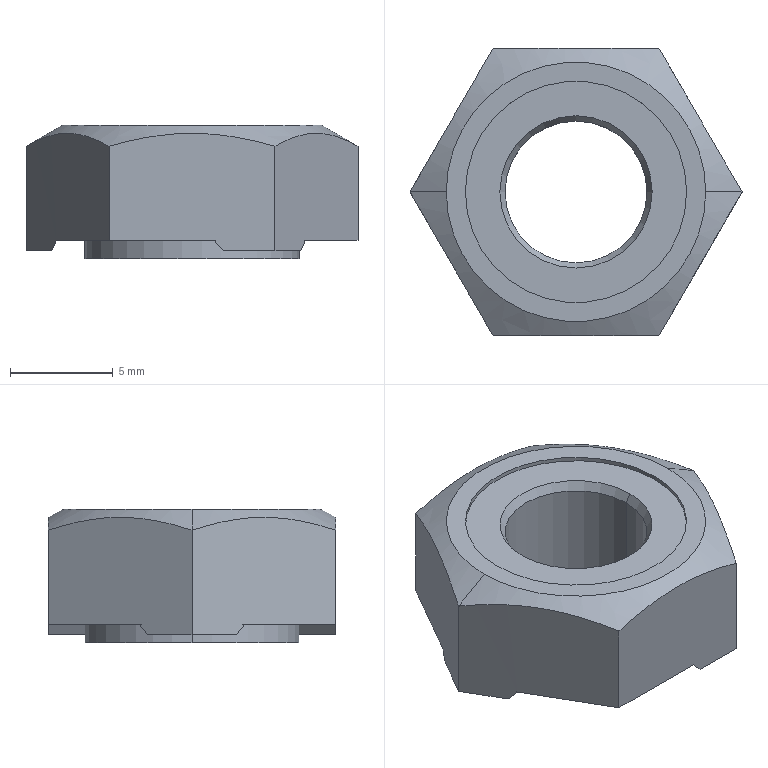Part | STEP file | VD-120102160011A_1_VD-SYL0-5601 | 1 solid | 28 faces | box 16.166 x 14 x 6.5 mm | volume 760.223 mm3 | plane 16 | cone 6 | cylinder 6 | commonest cylinder face diameters 6.917 x2 10.45 x2 10.77 x2
STEP:
#1=CARTESIAN_POINT('',(-3.458,0.,-0.6333));
#2=VERTEX_POINT('',#1);
#3=CARTESIAN_POINT('',(3.458,0.,-0.6333));
#4=VERTEX_POINT('',#3);
#5=CARTESIAN_POINT('',(0.,0.,-0.6333));
#6=DIRECTION('',(0.,0.,-1.));
#7=DIRECTION('',(-1.,0.,0.));
#8=AXIS2_PLACEMENT_3D('',#5,#6,#7);
#9=CIRCLE('',#8,3.458);
#10=EDGE_CURVE('',#2,#4,#9,.T.);
#11=ORIENTED_EDGE('',*,*,#10,.T.);
#12=CARTESIAN_POINT('',(3.709,0.,-0.2));
#13=VERTEX_POINT('',#12);
#14=CARTESIAN_POINT('',(3.709,0.,-0.2));
#15=DIRECTION('',(-0.5,0.,-0.866));
#16=VECTOR('',#15,1000.);
#17=LINE('',#14,#16);
#18=EDGE_CURVE('',#13,#4,#17,.T.);
#19=ORIENTED_EDGE('',*,*,#18,.F.);
#20=CARTESIAN_POINT('',(-3.709,0.,-0.2));
#21=VERTEX_POINT('',#20);
#22=CARTESIAN_POINT('',(0.,0.,-0.2));
#23=DIRECTION('',(0.,0.,-1.));
#24=DIRECTION('',(-1.,0.,0.));
#25=AXIS2_PLACEMENT_3D('',#22,#23,#24);
#26=CIRCLE('',#25,3.709);
#27=EDGE_CURVE('',#21,#13,#26,.T.);
#28=ORIENTED_EDGE('',*,*,#27,.F.);
#29=CARTESIAN_POINT('',(-3.709,0.,-0.2));
#30=DIRECTION('',(0.5,0.,-0.866));
#31=VECTOR('',#30,1000.);
#32=LINE('',#29,#31);
#33=EDGE_CURVE('',#21,#2,#32,.T.);
#34=ORIENTED_EDGE('',*,*,#33,.T.);
#35=EDGE_LOOP('',(#11,#19,#28,#34));
#36=FACE_OUTER_BOUND('',#35,.T.);
#37=CARTESIAN_POINT('',(0.,0.,-0.4167));
#38=DIRECTION('',(0.,0.,1.));
#39=DIRECTION('',(1.,0.,0.));
#40=AXIS2_PLACEMENT_3D('',#37,#38,#39);
#41=CONICAL_SURFACE('',#40,3.584,0.5236);
#42=ADVANCED_FACE('',(#36),#41,.F.);
#43=CARTESIAN_POINT('',(5.291,-4.835,-6.1));
#44=VERTEX_POINT('',#43);
#45=CARTESIAN_POINT('',(4.041,-7.,-6.1));
#46=VERTEX_POINT('',#45);
#47=CARTESIAN_POINT('',(5.291,-4.835,-6.1));
#48=DIRECTION('',(-0.5,-0.866,0.));
#49=VECTOR('',#48,1000.);
#50=LINE('',#47,#49);
#51=EDGE_CURVE('',#44,#46,#50,.T.);
#52=ORIENTED_EDGE('',*,*,#51,.T.);
#53=CARTESIAN_POINT('',(1.541,-7.,-6.1));
#54=VERTEX_POINT('',#53);
#55=CARTESIAN_POINT('',(4.041,-7.,-6.1));
#56=DIRECTION('',(-1.,0.,0.));
#57=VECTOR('',#56,1000.);
#58=LINE('',#55,#57);
#59=EDGE_CURVE('',#46,#54,#58,.T.);
#60=ORIENTED_EDGE('',*,*,#59,.T.);
#61=CARTESIAN_POINT('',(1.541,-7.,-6.1));
#62=DIRECTION('',(0.866,0.5,0.));
#63=VECTOR('',#62,1000.);
#64=LINE('',#61,#63);
#65=EDGE_CURVE('',#54,#44,#64,.T.);
#66=ORIENTED_EDGE('',*,*,#65,.T.);
#67=EDGE_LOOP('',(#52,#60,#66));
#68=FACE_OUTER_BOUND('',#67,.T.);
#69=CARTESIAN_POINT('',(4.041,-7.,-6.1));
#70=DIRECTION('',(0.,0.,-1.));
#71=DIRECTION('',(0.,-1.,0.));
#72=AXIS2_PLACEMENT_3D('',#69,#70,#71);
#73=PLANE('',#72);
#74=ADVANCED_FACE('',(#68),#73,.T.);
#75=CARTESIAN_POINT('',(1.075,-7.,-5.6));
#76=VERTEX_POINT('',#75);
#77=CARTESIAN_POINT('',(5.525,-4.431,-5.6));
#78=VERTEX_POINT('',#77);
#79=CARTESIAN_POINT('',(1.075,-7.,-5.6));
#80=DIRECTION('',(0.866,0.5,0.));
#81=VECTOR('',#80,1000.);
#82=LINE('',#79,#81);
#83=EDGE_CURVE('',#76,#78,#82,.T.);
#84=ORIENTED_EDGE('',*,*,#83,.T.);
#85=CARTESIAN_POINT('',(5.291,-4.835,-6.1));
#86=DIRECTION('',(0.341,0.5907,0.7313));
#87=VECTOR('',#86,1000.);
#88=LINE('',#85,#87);
#89=EDGE_CURVE('',#44,#78,#88,.T.);
#90=ORIENTED_EDGE('',*,*,#89,.F.);
#91=ORIENTED_EDGE('',*,*,#65,.F.);
#92=CARTESIAN_POINT('',(1.075,-7.,-5.6));
#93=DIRECTION('',(0.682,0.,-0.7313));
#94=VECTOR('',#93,1000.);
#95=LINE('',#92,#94);
#96=EDGE_CURVE('',#76,#54,#95,.T.);
#97=ORIENTED_EDGE('',*,*,#96,.F.);
#98=EDGE_LOOP('',(#84,#90,#91,#97));
#99=FACE_OUTER_BOUND('',#98,.T.);
#100=CARTESIAN_POINT('',(1.541,-7.,-6.1));
#101=DIRECTION('',(-0.4532,0.7849,-0.4226));
#102=DIRECTION('',(-0.682,0.,0.7313));
#103=AXIS2_PLACEMENT_3D('',#100,#101,#102);
#104=PLANE('',#103);
#105=ADVANCED_FACE('',(#99),#104,.T.);
#106=CARTESIAN_POINT('',(1.541,7.,-6.1));
#107=VERTEX_POINT('',#106);
#108=CARTESIAN_POINT('',(4.041,7.,-6.1));
#109=VERTEX_POINT('',#108);
#110=CARTESIAN_POINT('',(1.541,7.,-6.1));
#111=DIRECTION('',(1.,0.,0.));
#112=VECTOR('',#111,1000.);
#113=LINE('',#110,#112);
#114=EDGE_CURVE('',#107,#109,#113,.T.);
#115=ORIENTED_EDGE('',*,*,#114,.T.);
#116=CARTESIAN_POINT('',(5.291,4.835,-6.1));
#117=VERTEX_POINT('',#116);
#118=CARTESIAN_POINT('',(4.041,7.,-6.1));
#119=DIRECTION('',(0.5,-0.866,0.));
#120=VECTOR('',#119,1000.);
#121=LINE('',#118,#120);
#122=EDGE_CURVE('',#109,#117,#121,.T.);
#123=ORIENTED_EDGE('',*,*,#122,.T.);
#124=CARTESIAN_POINT('',(5.291,4.835,-6.1));
#125=DIRECTION('',(-0.866,0.5,0.));
#126=VECTOR('',#125,1000.);
#127=LINE('',#124,#126);
#128=EDGE_CURVE('',#117,#107,#127,.T.);
#129=ORIENTED_EDGE('',*,*,#128,.T.);
#130=EDGE_LOOP('',(#115,#123,#129));
#131=FACE_OUTER_BOUND('',#130,.T.);
#132=CARTESIAN_POINT('',(4.041,7.,-6.1));
#133=DIRECTION('',(0.,0.,-1.));
#134=DIRECTION('',(0.,-1.,0.));
#135=AXIS2_PLACEMENT_3D('',#132,#133,#134);
#136=PLANE('',#135);
#137=ADVANCED_FACE('',(#131),#136,.T.);
#138=CARTESIAN_POINT('',(1.075,7.,-5.6));
#139=VERTEX_POINT('',#138);
#140=CARTESIAN_POINT('',(5.525,4.431,-5.6));
#141=VERTEX_POINT('',#140);
#142=CARTESIAN_POINT('',(1.075,7.,-5.6));
#143=DIRECTION('',(0.866,-0.5,0.));
#144=VECTOR('',#143,1000.);
#145=LINE('',#142,#144);
#146=EDGE_CURVE('',#139,#141,#145,.T.);
#147=ORIENTED_EDGE('',*,*,#146,.F.);
#148=CARTESIAN_POINT('',(1.541,7.,-6.1));
#149=DIRECTION('',(-0.682,0.,0.7313));
#150=VECTOR('',#149,1000.);
#151=LINE('',#148,#150);
#152=EDGE_CURVE('',#107,#139,#151,.T.);
#153=ORIENTED_EDGE('',*,*,#152,.F.);
#154=ORIENTED_EDGE('',*,*,#128,.F.);
#155=CARTESIAN_POINT('',(5.291,4.835,-6.1));
#156=DIRECTION('',(0.341,-0.5907,0.7313));
#157=VECTOR('',#156,1000.);
#158=LINE('',#155,#157);
#159=EDGE_CURVE('',#117,#141,#158,.T.);
#160=ORIENTED_EDGE('',*,*,#159,.T.);
#161=EDGE_LOOP('',(#147,#153,#154,#160));
#162=FACE_OUTER_BOUND('',#161,.T.);
#163=CARTESIAN_POINT('',(5.291,4.835,-6.1));
#164=DIRECTION('',(-0.4532,-0.7849,-0.4226));
#165=DIRECTION('',(-0.866,0.5,0.));
#166=AXIS2_PLACEMENT_3D('',#163,#164,#165);
#167=PLANE('',#166);
#168=ADVANCED_FACE('',(#162),#167,.T.);
#169=CARTESIAN_POINT('',(-6.6,2.569,-5.6));
#170=VERTEX_POINT('',#169);
#171=CARTESIAN_POINT('',(-6.6,-2.569,-5.6));
#172=VERTEX_POINT('',#171);
#173=CARTESIAN_POINT('',(-6.6,2.569,-5.6));
#174=DIRECTION('',(0.,-1.,0.));
#175=VECTOR('',#174,1000.);
#176=LINE('',#173,#175);
#177=EDGE_CURVE('',#170,#172,#176,.T.);
#178=ORIENTED_EDGE('',*,*,#177,.T.);
#179=CARTESIAN_POINT('',(-6.833,-2.165,-6.1));
#180=VERTEX_POINT('',#179);
#181=CARTESIAN_POINT('',(-6.6,-2.569,-5.6));
#182=DIRECTION('',(-0.341,0.5907,-0.7313));
#183=VECTOR('',#182,1000.);
#184=LINE('',#181,#183);
#185=EDGE_CURVE('',#172,#180,#184,.T.);
#186=ORIENTED_EDGE('',*,*,#185,.T.);
#187=CARTESIAN_POINT('',(-6.833,2.165,-6.1));
#188=VERTEX_POINT('',#187);
#189=CARTESIAN_POINT('',(-6.833,2.165,-6.1));
#190=DIRECTION('',(0.,-1.,0.));
#191=VECTOR('',#190,1000.);
#192=LINE('',#189,#191);
#193=EDGE_CURVE('',#188,#180,#192,.T.);
#194=ORIENTED_EDGE('',*,*,#193,.F.);
#195=CARTESIAN_POINT('',(-6.833,2.165,-6.1));
#196=DIRECTION('',(0.341,0.5907,0.7313));
#197=VECTOR('',#196,1000.);
#198=LINE('',#195,#197);
#199=EDGE_CURVE('',#188,#170,#198,.T.);
#200=ORIENTED_EDGE('',*,*,#199,.T.);
#201=EDGE_LOOP('',(#178,#186,#194,#200));
#202=FACE_OUTER_BOUND('',#201,.T.);
#203=CARTESIAN_POINT('',(-6.833,2.165,-6.1));
#204=DIRECTION('',(0.9063,0.,-0.4226));
#205=DIRECTION('',(0.,-1.,0.));
#206=AXIS2_PLACEMENT_3D('',#203,#204,#205);
#207=PLANE('',#206);
#208=ADVANCED_FACE('',(#202),#207,.T.);
#209=CARTESIAN_POINT('',(-8.083,0.,-6.1));
#210=VERTEX_POINT('',#209);
#211=CARTESIAN_POINT('',(-6.833,-2.165,-6.1));
#212=DIRECTION('',(-0.5,0.866,0.));
#213=VECTOR('',#212,1000.);
#214=LINE('',#211,#213);
#215=EDGE_CURVE('',#180,#210,#214,.T.);
#216=ORIENTED_EDGE('',*,*,#215,.T.);
#217=CARTESIAN_POINT('',(-8.083,0.,-6.1));
#218=DIRECTION('',(0.5,0.866,0.));
#219=VECTOR('',#218,1000.);
#220=LINE('',#217,#219);
#221=EDGE_CURVE('',#210,#188,#220,.T.);
#222=ORIENTED_EDGE('',*,*,#221,.T.);
#223=ORIENTED_EDGE('',*,*,#193,.T.);
#224=EDGE_LOOP('',(#216,#222,#223));
#225=FACE_OUTER_BOUND('',#224,.T.);
#226=CARTESIAN_POINT('',(-8.083,0.,-6.1));
#227=DIRECTION('',(0.,0.,-1.));
#228=DIRECTION('',(0.,-1.,0.));
#229=AXIS2_PLACEMENT_3D('',#226,#227,#228);
#230=PLANE('',#229);
#231=ADVANCED_FACE('',(#225),#230,.T.);
#232=CARTESIAN_POINT('',(-4.041,7.,-1.021));
#233=VERTEX_POINT('',#232);
#234=CARTESIAN_POINT('',(-4.041,7.,-5.6));
#235=VERTEX_POINT('',#234);
#236=CARTESIAN_POINT('',(-4.041,7.,-1.021));
#237=DIRECTION('',(0.,0.,-1.));
#238=VECTOR('',#237,1000.);
#239=LINE('',#236,#238);
#240=EDGE_CURVE('',#233,#235,#239,.T.);
#241=ORIENTED_EDGE('',*,*,#240,.T.);
#242=CARTESIAN_POINT('',(-6.6,2.569,-5.6));
#243=DIRECTION('',(0.5,0.866,0.));
#244=VECTOR('',#243,1000.);
#245=LINE('',#242,#244);
#246=EDGE_CURVE('',#170,#235,#245,.T.);
#247=ORIENTED_EDGE('',*,*,#246,.F.);
#248=ORIENTED_EDGE('',*,*,#199,.F.);
#249=ORIENTED_EDGE('',*,*,#221,.F.);
#250=CARTESIAN_POINT('',(-8.083,0.,-1.021));
#251=VERTEX_POINT('',#250);
#252=CARTESIAN_POINT('',(-8.083,0.,-6.1));
#253=DIRECTION('',(0.,0.,1.));
#254=VECTOR('',#253,1000.);
#255=LINE('',#252,#254);
#256=EDGE_CURVE('',#210,#251,#255,.T.);
#257=ORIENTED_EDGE('',*,*,#256,.T.);
#258=CARTESIAN_POINT('',(-4.041,7.,-1.021));
#259=CARTESIAN_POINT('',(-4.218,6.695,-0.9189));
#260=CARTESIAN_POINT('',(-4.39,6.396,-0.8294));
#261=CARTESIAN_POINT('',(-4.644,5.955,-0.7134));
#262=CARTESIAN_POINT('',(-4.729,5.809,-0.6778));
#263=CARTESIAN_POINT('',(-4.855,5.591,-0.629));
#264=CARTESIAN_POINT('',(-4.897,5.519,-0.6134));
#265=CARTESIAN_POINT('',(-4.98,5.374,-0.5839));
#266=CARTESIAN_POINT('',(-5.021,5.303,-0.5702));
#267=CARTESIAN_POINT('',(-5.404,4.64,-0.449));
#268=CARTESIAN_POINT('',(-5.737,4.063,-0.3948));
#269=CARTESIAN_POINT('',(-6.234,3.203,-0.3958));
#270=CARTESIAN_POINT('',(-6.399,2.917,-0.4097));
#271=CARTESIAN_POINT('',(-6.648,2.485,-0.4507));
#272=CARTESIAN_POINT('',(-6.731,2.341,-0.4676));
#273=CARTESIAN_POINT('',(-6.857,2.124,-0.498));
#274=CARTESIAN_POINT('',(-6.898,2.052,-0.509));
#275=CARTESIAN_POINT('',(-6.982,1.906,-0.5326));
#276=CARTESIAN_POINT('',(-7.025,1.832,-0.5455));
#277=CARTESIAN_POINT('',(-7.399,1.185,-0.6644));
#278=CARTESIAN_POINT('',(-7.732,0.6069,-0.8184));
#279=CARTESIAN_POINT('',(-8.083,0.,-1.021));
#280=B_SPLINE_CURVE_WITH_KNOTS('',3,(#258,#259,#260,#261,#262,#263,#264,#265,#266,#267,#268,#269,#270,#271,#272,#273,#274,#275,#276,#277,#278,#279),.UNSPECIFIED.,.F.,.F.,(4,2,2,2,2,2,2,2,2,2,4),(0.,0.125,0.1875,0.2187,0.25,0.5,0.625,0.6875,0.7188,0.75,1.),.UNSPECIFIED.);
#281=EDGE_CURVE('',#233,#251,#280,.T.);
#282=ORIENTED_EDGE('',*,*,#281,.F.);
#283=EDGE_LOOP('',(#241,#247,#248,#249,#257,#282));
#284=FACE_OUTER_BOUND('',#283,.T.);
#285=CARTESIAN_POINT('',(-4.041,7.,-6.5));
#286=DIRECTION('',(-0.866,0.5,0.));
#287=DIRECTION('',(0.,0.,1.));
#288=AXIS2_PLACEMENT_3D('',#285,#286,#287);
#289=PLANE('',#288);
#290=ADVANCED_FACE('',(#284),#289,.T.);
#291=CARTESIAN_POINT('',(4.041,7.,-1.021));
#292=VERTEX_POINT('',#291);
#293=CARTESIAN_POINT('',(4.041,7.,-1.021));
#294=DIRECTION('',(0.,0.,-1.));
#295=VECTOR('',#294,1000.);
#296=LINE('',#293,#295);
#297=EDGE_CURVE('',#292,#109,#296,.T.);
#298=ORIENTED_EDGE('',*,*,#297,.T.);
#299=ORIENTED_EDGE('',*,*,#114,.F.);
#300=ORIENTED_EDGE('',*,*,#152,.T.);
#301=CARTESIAN_POINT('',(1.075,7.,-5.6));
#302=DIRECTION('',(-1.,0.,0.));
#303=VECTOR('',#302,1000.);
#304=LINE('',#301,#303);
#305=EDGE_CURVE('',#139,#235,#304,.T.);
#306=ORIENTED_EDGE('',*,*,#305,.T.);
#307=ORIENTED_EDGE('',*,*,#240,.F.);
#308=CARTESIAN_POINT('',(4.041,7.,-1.021));
#309=CARTESIAN_POINT('',(3.689,7.,-0.9189));
#310=CARTESIAN_POINT('',(3.345,7.,-0.8294));
#311=CARTESIAN_POINT('',(2.835,7.,-0.7134));
#312=CARTESIAN_POINT('',(2.667,7.,-0.6778));
#313=CARTESIAN_POINT('',(2.415,7.,-0.629));
#314=CARTESIAN_POINT('',(2.331,7.,-0.6134));
#315=CARTESIAN_POINT('',(2.164,7.,-0.5839));
#316=CARTESIAN_POINT('',(2.082,7.,-0.5702));
#317=CARTESIAN_POINT('',(1.316,7.,-0.449));
#318=CARTESIAN_POINT('',(0.6504,7.,-0.3948));
#319=CARTESIAN_POINT('',(-0.3433,7.,-0.3958));
#320=CARTESIAN_POINT('',(-0.6728,7.,-0.4097));
#321=CARTESIAN_POINT('',(-1.172,7.,-0.4507));
#322=CARTESIAN_POINT('',(-1.338,7.,-0.4676));
#323=CARTESIAN_POINT('',(-1.589,7.,-0.498));
#324=CARTESIAN_POINT('',(-1.673,7.,-0.509));
#325=CARTESIAN_POINT('',(-1.84,7.,-0.5326));
#326=CARTESIAN_POINT('',(-1.926,7.,-0.5455));
#327=CARTESIAN_POINT('',(-2.673,7.,-0.6644));
#328=CARTESIAN_POINT('',(-3.341,7.,-0.8184));
#329=CARTESIAN_POINT('',(-4.041,7.,-1.021));
#330=B_SPLINE_CURVE_WITH_KNOTS('',3,(#308,#309,#310,#311,#312,#313,#314,#315,#316,#317,#318,#319,#320,#321,#322,#323,#324,#325,#326,#327,#328,#329),.UNSPECIFIED.,.F.,.F.,(4,2,2,2,2,2,2,2,2,2,4),(0.,0.125,0.1875,0.2188,0.25,0.5,0.625,0.6875,0.7188,0.75,1.),.UNSPECIFIED.);
#331=EDGE_CURVE('',#292,#233,#330,.T.);
#332=ORIENTED_EDGE('',*,*,#331,.F.);
#333=EDGE_LOOP('',(#298,#299,#300,#306,#307,#332));
#334=FACE_OUTER_BOUND('',#333,.T.);
#335=CARTESIAN_POINT('',(4.041,7.,-6.5));
#336=DIRECTION('',(0.,1.,0.));
#337=DIRECTION('',(1.,0.,0.));
#338=AXIS2_PLACEMENT_3D('',#335,#336,#337);
#339=PLANE('',#338);
#340=ADVANCED_FACE('',(#334),#339,.T.);
#341=CARTESIAN_POINT('',(8.083,0.,-1.021));
#342=VERTEX_POINT('',#341);
#343=CARTESIAN_POINT('',(8.083,0.,-5.6));
#344=VERTEX_POINT('',#343);
#345=CARTESIAN_POINT('',(8.083,0.,-1.021));
#346=DIRECTION('',(0.,0.,-1.));
#347=VECTOR('',#346,1000.);
#348=LINE('',#345,#347);
#349=EDGE_CURVE('',#342,#344,#348,.T.);
#350=ORIENTED_EDGE('',*,*,#349,.T.);
#351=CARTESIAN_POINT('',(5.525,4.431,-5.6));
#352=DIRECTION('',(0.5,-0.866,0.));
#353=VECTOR('',#352,1000.);
#354=LINE('',#351,#353);
#355=EDGE_CURVE('',#141,#344,#354,.T.);
#356=ORIENTED_EDGE('',*,*,#355,.F.);
#357=ORIENTED_EDGE('',*,*,#159,.F.);
#358=ORIENTED_EDGE('',*,*,#122,.F.);
#359=ORIENTED_EDGE('',*,*,#297,.F.);
#360=CARTESIAN_POINT('',(8.083,0.,-1.021));
#361=CARTESIAN_POINT('',(7.907,0.3053,-0.9189));
#362=CARTESIAN_POINT('',(7.734,0.6035,-0.8294));
#363=CARTESIAN_POINT('',(7.48,1.044,-0.7134));
#364=CARTESIAN_POINT('',(7.395,1.19,-0.6778));
#365=CARTESIAN_POINT('',(7.27,1.409,-0.629));
#366=CARTESIAN_POINT('',(7.228,1.481,-0.6134));
#367=CARTESIAN_POINT('',(7.144,1.626,-0.5839));
#368=CARTESIAN_POINT('',(7.103,1.697,-0.5702));
#369=CARTESIAN_POINT('',(6.72,2.36,-0.449));
#370=CARTESIAN_POINT('',(6.387,2.937,-0.3948));
#371=CARTESIAN_POINT('',(5.89,3.797,-0.3958));
#372=CARTESIAN_POINT('',(5.726,4.083,-0.4097));
#373=CARTESIAN_POINT('',(5.476,4.515,-0.4507));
#374=CARTESIAN_POINT('',(5.393,4.659,-0.4676));
#375=CARTESIAN_POINT('',(5.268,4.876,-0.498));
#376=CARTESIAN_POINT('',(5.226,4.948,-0.509));
#377=CARTESIAN_POINT('',(5.142,5.094,-0.5326));
#378=CARTESIAN_POINT('',(5.099,5.168,-0.5455));
#379=CARTESIAN_POINT('',(4.726,5.815,-0.6644));
#380=CARTESIAN_POINT('',(4.392,6.393,-0.8184));
#381=CARTESIAN_POINT('',(4.041,7.,-1.021));
#382=B_SPLINE_CURVE_WITH_KNOTS('',3,(#360,#361,#362,#363,#364,#365,#366,#367,#368,#369,#370,#371,#372,#373,#374,#375,#376,#377,#378,#379,#380,#381),.UNSPECIFIED.,.F.,.F.,(4,2,2,2,2,2,2,2,2,2,4),(0.,0.125,0.1875,0.2188,0.25,0.5,0.625,0.6875,0.7188,0.75,1.),.UNSPECIFIED.);
#383=EDGE_CURVE('',#342,#292,#382,.T.);
#384=ORIENTED_EDGE('',*,*,#383,.F.);
#385=EDGE_LOOP('',(#350,#356,#357,#358,#359,#384));
#386=FACE_OUTER_BOUND('',#385,.T.);
#387=CARTESIAN_POINT('',(8.083,0.,-6.5));
#388=DIRECTION('',(0.866,0.5,0.));
#389=DIRECTION('',(0.,0.,-1.));
#390=AXIS2_PLACEMENT_3D('',#387,#388,#389);
#391=PLANE('',#390);
#392=ADVANCED_FACE('',(#386),#391,.T.);
#393=CARTESIAN_POINT('',(4.041,-7.,-1.021));
#394=VERTEX_POINT('',#393);
#395=CARTESIAN_POINT('',(4.041,-7.,-1.021));
#396=DIRECTION('',(0.,0.,-1.));
#397=VECTOR('',#396,1000.);
#398=LINE('',#395,#397);
#399=EDGE_CURVE('',#394,#46,#398,.T.);
#400=ORIENTED_EDGE('',*,*,#399,.T.);
#401=ORIENTED_EDGE('',*,*,#51,.F.);
#402=ORIENTED_EDGE('',*,*,#89,.T.);
#403=CARTESIAN_POINT('',(8.083,0.,-5.6));
#404=DIRECTION('',(-0.5,-0.866,0.));
#405=VECTOR('',#404,1000.);
#406=LINE('',#403,#405);
#407=EDGE_CURVE('',#344,#78,#406,.T.);
#408=ORIENTED_EDGE('',*,*,#407,.F.);
#409=ORIENTED_EDGE('',*,*,#349,.F.);
#410=CARTESIAN_POINT('',(4.041,-7.,-1.021));
#411=CARTESIAN_POINT('',(4.218,-6.695,-0.9189));
#412=CARTESIAN_POINT('',(4.39,-6.396,-0.8294));
#413=CARTESIAN_POINT('',(4.644,-5.955,-0.7134));
#414=CARTESIAN_POINT('',(4.729,-5.809,-0.6778));
#415=CARTESIAN_POINT('',(4.855,-5.591,-0.629));
#416=CARTESIAN_POINT('',(4.897,-5.519,-0.6134));
#417=CARTESIAN_POINT('',(4.98,-5.374,-0.5839));
#418=CARTESIAN_POINT('',(5.021,-5.303,-0.5702));
#419=CARTESIAN_POINT('',(5.404,-4.64,-0.449));
#420=CARTESIAN_POINT('',(5.737,-4.063,-0.3948));
#421=CARTESIAN_POINT('',(6.234,-3.203,-0.3958));
#422=CARTESIAN_POINT('',(6.399,-2.917,-0.4097));
#423=CARTESIAN_POINT('',(6.648,-2.485,-0.4507));
#424=CARTESIAN_POINT('',(6.731,-2.341,-0.4676));
#425=CARTESIAN_POINT('',(6.857,-2.124,-0.498));
#426=CARTESIAN_POINT('',(6.898,-2.052,-0.509));
#427=CARTESIAN_POINT('',(6.982,-1.906,-0.5326));
#428=CARTESIAN_POINT('',(7.025,-1.832,-0.5455));
#429=CARTESIAN_POINT('',(7.399,-1.185,-0.6644));
#430=CARTESIAN_POINT('',(7.732,-0.6069,-0.8184));
#431=CARTESIAN_POINT('',(8.083,0.,-1.021));
#432=B_SPLINE_CURVE_WITH_KNOTS('',3,(#410,#411,#412,#413,#414,#415,#416,#417,#418,#419,#420,#421,#422,#423,#424,#425,#426,#427,#428,#429,#430,#431),.UNSPECIFIED.,.F.,.F.,(4,2,2,2,2,2,2,2,2,2,4),(0.,0.125,0.1875,0.2188,0.25,0.5,0.625,0.6875,0.7188,0.75,1.),.UNSPECIFIED.);
#433=EDGE_CURVE('',#394,#342,#432,.T.);
#434=ORIENTED_EDGE('',*,*,#433,.F.);
#435=EDGE_LOOP('',(#400,#401,#402,#408,#409,#434));
#436=FACE_OUTER_BOUND('',#435,.T.);
#437=CARTESIAN_POINT('',(4.041,-7.,-6.5));
#438=DIRECTION('',(0.866,-0.5,0.));
#439=DIRECTION('',(0.,0.,-1.));
#440=AXIS2_PLACEMENT_3D('',#437,#438,#439);
#441=PLANE('',#440);
#442=ADVANCED_FACE('',(#436),#441,.T.);
#443=CARTESIAN_POINT('',(-4.041,-7.,-1.021));
#444=VERTEX_POINT('',#443);
#445=CARTESIAN_POINT('',(-4.041,-7.,-5.6));
#446=VERTEX_POINT('',#445);
#447=CARTESIAN_POINT('',(-4.041,-7.,-1.021));
#448=DIRECTION('',(0.,0.,-1.));
#449=VECTOR('',#448,1000.);
#450=LINE('',#447,#449);
#451=EDGE_CURVE('',#444,#446,#450,.T.);
#452=ORIENTED_EDGE('',*,*,#451,.T.);
#453=CARTESIAN_POINT('',(-4.041,-7.,-5.6));
#454=DIRECTION('',(1.,0.,0.));
#455=VECTOR('',#454,1000.);
#456=LINE('',#453,#455);
#457=EDGE_CURVE('',#446,#76,#456,.T.);
#458=ORIENTED_EDGE('',*,*,#457,.T.);
#459=ORIENTED_EDGE('',*,*,#96,.T.);
#460=ORIENTED_EDGE('',*,*,#59,.F.);
#461=ORIENTED_EDGE('',*,*,#399,.F.);
#462=CARTESIAN_POINT('',(-4.041,-7.,-1.021));
#463=CARTESIAN_POINT('',(-3.689,-7.,-0.9189));
#464=CARTESIAN_POINT('',(-3.345,-7.,-0.8294));
#465=CARTESIAN_POINT('',(-2.835,-7.,-0.7134));
#466=CARTESIAN_POINT('',(-2.667,-7.,-0.6778));
#467=CARTESIAN_POINT('',(-2.415,-7.,-0.629));
#468=CARTESIAN_POINT('',(-2.331,-7.,-0.6134));
#469=CARTESIAN_POINT('',(-2.164,-7.,-0.5839));
#470=CARTESIAN_POINT('',(-2.082,-7.,-0.5702));
#471=CARTESIAN_POINT('',(-1.316,-7.,-0.449));
#472=CARTESIAN_POINT('',(-0.6504,-7.,-0.3948));
#473=CARTESIAN_POINT('',(0.3433,-7.,-0.3958));
#474=CARTESIAN_POINT('',(0.6728,-7.,-0.4097));
#475=CARTESIAN_POINT('',(1.172,-7.,-0.4507));
#476=CARTESIAN_POINT('',(1.338,-7.,-0.4676));
#477=CARTESIAN_POINT('',(1.589,-7.,-0.498));
#478=CARTESIAN_POINT('',(1.673,-7.,-0.509));
#479=CARTESIAN_POINT('',(1.84,-7.,-0.5326));
#480=CARTESIAN_POINT('',(1.926,-7.,-0.5455));
#481=CARTESIAN_POINT('',(2.673,-7.,-0.6644));
#482=CARTESIAN_POINT('',(3.341,-7.,-0.8184));
#483=CARTESIAN_POINT('',(4.041,-7.,-1.021));
#484=B_SPLINE_CURVE_WITH_KNOTS('',3,(#462,#463,#464,#465,#466,#467,#468,#469,#470,#471,#472,#473,#474,#475,#476,#477,#478,#479,#480,#481,#482,#483),.UNSPECIFIED.,.F.,.F.,(4,2,2,2,2,2,2,2,2,2,4),(0.,0.125,0.1875,0.2188,0.25,0.5,0.625,0.6875,0.7188,0.75,1.),.UNSPECIFIED.);
#485=EDGE_CURVE('',#444,#394,#484,.T.);
#486=ORIENTED_EDGE('',*,*,#485,.F.);
#487=EDGE_LOOP('',(#452,#458,#459,#460,#461,#486));
#488=FACE_OUTER_BOUND('',#487,.T.);
#489=CARTESIAN_POINT('',(-4.041,-7.,-6.5));
#490=DIRECTION('',(0.,-1.,0.));
#491=DIRECTION('',(0.,0.,-1.));
#492=AXIS2_PLACEMENT_3D('',#489,#490,#491);
#493=PLANE('',#492);
#494=ADVANCED_FACE('',(#488),#493,.T.);
#495=CARTESIAN_POINT('',(5.225,0.,-5.6));
#496=VERTEX_POINT('',#495);
#497=CARTESIAN_POINT('',(-5.225,0.,-5.6));
#498=VERTEX_POINT('',#497);
#499=CARTESIAN_POINT('',(0.,0.,-5.6));
#500=DIRECTION('',(0.,0.,1.));
#501=DIRECTION('',(1.,0.,0.));
#502=AXIS2_PLACEMENT_3D('',#499,#500,#501);
#503=CIRCLE('',#502,5.225);
#504=EDGE_CURVE('',#496,#498,#503,.T.);
#505=ORIENTED_EDGE('',*,*,#504,.T.);
#506=CARTESIAN_POINT('',(0.,0.,-5.6));
#507=DIRECTION('',(0.,0.,1.));
#508=DIRECTION('',(-1.,0.,0.));
#509=AXIS2_PLACEMENT_3D('',#506,#507,#508);
#510=CIRCLE('',#509,5.225);
#511=EDGE_CURVE('',#498,#496,#510,.T.);
#512=ORIENTED_EDGE('',*,*,#511,.T.);
#513=EDGE_LOOP('',(#505,#512));
#514=FACE_BOUND('',#513,.T.);
#515=CARTESIAN_POINT('',(-4.041,-7.,-5.6));
#516=DIRECTION('',(-0.5,0.866,0.));
#517=VECTOR('',#516,1000.);
#518=LINE('',#515,#517);
#519=EDGE_CURVE('',#446,#172,#518,.T.);
#520=ORIENTED_EDGE('',*,*,#519,.T.);
#521=ORIENTED_EDGE('',*,*,#177,.F.);
#522=ORIENTED_EDGE('',*,*,#246,.T.);
#523=ORIENTED_EDGE('',*,*,#305,.F.);
#524=ORIENTED_EDGE('',*,*,#146,.T.);
#525=ORIENTED_EDGE('',*,*,#355,.T.);
#526=ORIENTED_EDGE('',*,*,#407,.T.);
#527=ORIENTED_EDGE('',*,*,#83,.F.);
#528=ORIENTED_EDGE('',*,*,#457,.F.);
#529=EDGE_LOOP('',(#520,#521,#522,#523,#524,#525,#526,#527,#528));
#530=FACE_OUTER_BOUND('',#529,.T.);
#531=CARTESIAN_POINT('',(0.,0.,-5.6));
#532=DIRECTION('',(0.,0.,-1.));
#533=DIRECTION('',(0.,-1.,0.));
#534=AXIS2_PLACEMENT_3D('',#531,#532,#533);
#535=PLANE('',#534);
#536=ADVANCED_FACE('',(#514,#530),#535,.T.);
#537=CARTESIAN_POINT('',(5.225,0.,-6.5));
#538=VERTEX_POINT('',#537);
#539=CARTESIAN_POINT('',(5.225,0.,-6.5));
#540=DIRECTION('',(0.,0.,1.));
#541=VECTOR('',#540,1000.);
#542=LINE('',#539,#541);
#543=EDGE_CURVE('',#538,#496,#542,.T.);
#544=ORIENTED_EDGE('',*,*,#543,.F.);
#545=CARTESIAN_POINT('',(-5.225,0.,-6.5));
#546=VERTEX_POINT('',#545);
#547=CARTESIAN_POINT('',(0.,0.,-6.5));
#548=DIRECTION('',(0.,0.,-1.));
#549=DIRECTION('',(-1.,0.,0.));
#550=AXIS2_PLACEMENT_3D('',#547,#548,#549);
#551=CIRCLE('',#550,5.225);
#552=EDGE_CURVE('',#546,#538,#551,.T.);
#553=ORIENTED_EDGE('',*,*,#552,.F.);
#554=CARTESIAN_POINT('',(-5.225,0.,-6.5));
#555=DIRECTION('',(0.,0.,1.));
#556=VECTOR('',#555,1000.);
#557=LINE('',#554,#556);
#558=EDGE_CURVE('',#546,#498,#557,.T.);
#559=ORIENTED_EDGE('',*,*,#558,.T.);
#560=ORIENTED_EDGE('',*,*,#504,.F.);
#561=EDGE_LOOP('',(#544,#553,#559,#560));
#562=FACE_OUTER_BOUND('',#561,.T.);
#563=CARTESIAN_POINT('',(0.,0.,-5.6));
#564=DIRECTION('',(0.,0.,-1.));
#565=DIRECTION('',(-1.,0.,0.));
#566=AXIS2_PLACEMENT_3D('',#563,#564,#565);
#567=CYLINDRICAL_SURFACE('',#566,5.225);
#568=ADVANCED_FACE('',(#562),#567,.T.);
#569=ORIENTED_EDGE('',*,*,#511,.F.);
#570=ORIENTED_EDGE('',*,*,#558,.F.);
#571=CARTESIAN_POINT('',(0.,0.,-6.5));
#572=DIRECTION('',(0.,0.,-1.));
#573=DIRECTION('',(1.,0.,0.));
#574=AXIS2_PLACEMENT_3D('',#571,#572,#573);
#575=CIRCLE('',#574,5.225);
#576=EDGE_CURVE('',#538,#546,#575,.T.);
#577=ORIENTED_EDGE('',*,*,#576,.F.);
#578=ORIENTED_EDGE('',*,*,#543,.T.);
#579=EDGE_LOOP('',(#569,#570,#577,#578));
#580=FACE_OUTER_BOUND('',#579,.T.);
#581=CARTESIAN_POINT('',(0.,0.,-5.6));
#582=DIRECTION('',(0.,0.,-1.));
#583=DIRECTION('',(-1.,0.,0.));
#584=AXIS2_PLACEMENT_3D('',#581,#582,#583);
#585=CYLINDRICAL_SURFACE('',#584,5.225);
#586=ADVANCED_FACE('',(#580),#585,.T.);
#587=CARTESIAN_POINT('',(3.892,0.,-6.5));
#588=VERTEX_POINT('',#587);
#589=CARTESIAN_POINT('',(-3.892,0.,-6.5));
#590=VERTEX_POINT('',#589);
#591=CARTESIAN_POINT('',(0.,0.,-6.5));
#592=DIRECTION('',(0.,0.,1.));
#593=DIRECTION('',(1.,0.,0.));
#594=AXIS2_PLACEMENT_3D('',#591,#592,#593);
#595=CIRCLE('',#594,3.892);
#596=EDGE_CURVE('',#588,#590,#595,.T.);
#597=ORIENTED_EDGE('',*,*,#596,.T.);
#598=CARTESIAN_POINT('',(0.,0.,-6.5));
#599=DIRECTION('',(0.,0.,1.));
#600=DIRECTION('',(-1.,0.,0.));
#601=AXIS2_PLACEMENT_3D('',#598,#599,#600);
#602=CIRCLE('',#601,3.892);
#603=EDGE_CURVE('',#590,#588,#602,.T.);
#604=ORIENTED_EDGE('',*,*,#603,.T.);
#605=EDGE_LOOP('',(#597,#604));
#606=FACE_BOUND('',#605,.T.);
#607=ORIENTED_EDGE('',*,*,#552,.T.);
#608=ORIENTED_EDGE('',*,*,#576,.T.);
#609=EDGE_LOOP('',(#607,#608));
#610=FACE_OUTER_BOUND('',#609,.T.);
#611=CARTESIAN_POINT('',(-4.041,-7.,-6.5));
#612=DIRECTION('',(0.,0.,-1.));
#613=DIRECTION('',(0.,-1.,0.));
#614=AXIS2_PLACEMENT_3D('',#611,#612,#613);
#615=PLANE('',#614);
#616=ADVANCED_FACE('',(#606,#610),#615,.T.);
#617=CARTESIAN_POINT('',(3.459,0.,-6.25));
#618=VERTEX_POINT('',#617);
#619=CARTESIAN_POINT('',(3.892,0.,-6.5));
#620=DIRECTION('',(-0.866,0.,0.5));
#621=VECTOR('',#620,1000.);
#622=LINE('',#619,#621);
#623=EDGE_CURVE('',#588,#618,#622,.T.);
#624=ORIENTED_EDGE('',*,*,#623,.F.);
#625=ORIENTED_EDGE('',*,*,#603,.F.);
#626=CARTESIAN_POINT('',(-3.459,0.,-6.25));
#627=VERTEX_POINT('',#626);
#628=CARTESIAN_POINT('',(-3.892,0.,-6.5));
#629=DIRECTION('',(0.866,0.,0.5));
#630=VECTOR('',#629,1000.);
#631=LINE('',#628,#630);
#632=EDGE_CURVE('',#590,#627,#631,.T.);
#633=ORIENTED_EDGE('',*,*,#632,.T.);
#634=CARTESIAN_POINT('',(0.,0.,-6.25));
#635=DIRECTION('',(0.,0.,1.));
#636=DIRECTION('',(-1.,0.,0.));
#637=AXIS2_PLACEMENT_3D('',#634,#635,#636);
#638=CIRCLE('',#637,3.459);
#639=EDGE_CURVE('',#627,#618,#638,.T.);
#640=ORIENTED_EDGE('',*,*,#639,.T.);
#641=EDGE_LOOP('',(#624,#625,#633,#640));
#642=FACE_OUTER_BOUND('',#641,.T.);
#643=CARTESIAN_POINT('',(0.,0.,-6.375));
#644=DIRECTION('',(0.,0.,-1.));
#645=DIRECTION('',(-1.,0.,0.));
#646=AXIS2_PLACEMENT_3D('',#643,#644,#645);
#647=CONICAL_SURFACE('',#646,3.675,1.047);
#648=ADVANCED_FACE('',(#642),#647,.F.);
#649=CARTESIAN_POINT('',(0.,0.,-6.25));
#650=DIRECTION('',(0.,0.,1.));
#651=DIRECTION('',(1.,0.,0.));
#652=AXIS2_PLACEMENT_3D('',#649,#650,#651);
#653=CIRCLE('',#652,3.459);
#654=EDGE_CURVE('',#618,#627,#653,.T.);
#655=ORIENTED_EDGE('',*,*,#654,.T.);
#656=ORIENTED_EDGE('',*,*,#632,.F.);
#657=ORIENTED_EDGE('',*,*,#596,.F.);
#658=ORIENTED_EDGE('',*,*,#623,.T.);
#659=EDGE_LOOP('',(#655,#656,#657,#658));
#660=FACE_OUTER_BOUND('',#659,.T.);
#661=CARTESIAN_POINT('',(0.,0.,-6.375));
#662=DIRECTION('',(0.,0.,-1.));
#663=DIRECTION('',(-1.,0.,0.));
#664=AXIS2_PLACEMENT_3D('',#661,#662,#663);
#665=CONICAL_SURFACE('',#664,3.675,1.047);
#666=ADVANCED_FACE('',(#660),#665,.F.);
#667=ORIENTED_EDGE('',*,*,#10,.F.);
#668=CARTESIAN_POINT('',(-3.459,0.,-6.25));
#669=DIRECTION('',(0.,0.,1.));
#670=VECTOR('',#669,1000.);
#671=LINE('',#668,#670);
#672=EDGE_CURVE('',#627,#2,#671,.T.);
#673=ORIENTED_EDGE('',*,*,#672,.F.);
#674=ORIENTED_EDGE('',*,*,#654,.F.);
#675=CARTESIAN_POINT('',(3.459,0.,-6.25));
#676=DIRECTION('',(0.,0.,1.));
#677=VECTOR('',#676,1000.);
#678=LINE('',#675,#677);
#679=EDGE_CURVE('',#618,#4,#678,.T.);
#680=ORIENTED_EDGE('',*,*,#679,.T.);
#681=EDGE_LOOP('',(#667,#673,#674,#680));
#682=FACE_OUTER_BOUND('',#681,.T.);
#683=CARTESIAN_POINT('',(0.,0.,0.));
#684=DIRECTION('',(0.,0.,-1.));
#685=DIRECTION('',(-1.,0.,0.));
#686=AXIS2_PLACEMENT_3D('',#683,#684,#685);
#687=CYLINDRICAL_SURFACE('',#686,3.459);
#688=ADVANCED_FACE('',(#682),#687,.F.);
#689=ORIENTED_EDGE('',*,*,#679,.F.);
#690=ORIENTED_EDGE('',*,*,#639,.F.);
#691=ORIENTED_EDGE('',*,*,#672,.T.);
#692=CARTESIAN_POINT('',(0.,0.,-0.6333));
#693=DIRECTION('',(0.,0.,-1.));
#694=DIRECTION('',(1.,0.,0.));
#695=AXIS2_PLACEMENT_3D('',#692,#693,#694);
#696=CIRCLE('',#695,3.458);
#697=EDGE_CURVE('',#4,#2,#696,.T.);
#698=ORIENTED_EDGE('',*,*,#697,.F.);
#699=EDGE_LOOP('',(#689,#690,#691,#698));
#700=FACE_OUTER_BOUND('',#699,.T.);
#701=CARTESIAN_POINT('',(0.,0.,0.));
#702=DIRECTION('',(0.,0.,-1.));
#703=DIRECTION('',(-1.,0.,0.));
#704=AXIS2_PLACEMENT_3D('',#701,#702,#703);
#705=CYLINDRICAL_SURFACE('',#704,3.459);
#706=ADVANCED_FACE('',(#700),#705,.F.);
#707=ORIENTED_EDGE('',*,*,#33,.F.);
#708=CARTESIAN_POINT('',(0.,0.,-0.2));
#709=DIRECTION('',(0.,0.,-1.));
#710=DIRECTION('',(1.,0.,0.));
#711=AXIS2_PLACEMENT_3D('',#708,#709,#710);
#712=CIRCLE('',#711,3.709);
#713=EDGE_CURVE('',#13,#21,#712,.T.);
#714=ORIENTED_EDGE('',*,*,#713,.F.);
#715=ORIENTED_EDGE('',*,*,#18,.T.);
#716=ORIENTED_EDGE('',*,*,#697,.T.);
#717=EDGE_LOOP('',(#707,#714,#715,#716));
#718=FACE_OUTER_BOUND('',#717,.T.);
#719=CARTESIAN_POINT('',(0.,0.,-0.4167));
#720=DIRECTION('',(0.,0.,1.));
#721=DIRECTION('',(1.,0.,0.));
#722=AXIS2_PLACEMENT_3D('',#719,#720,#721);
#723=CONICAL_SURFACE('',#722,3.584,0.5236);
#724=ADVANCED_FACE('',(#718),#723,.F.);
#725=ORIENTED_EDGE('',*,*,#27,.T.);
#726=ORIENTED_EDGE('',*,*,#713,.T.);
#727=EDGE_LOOP('',(#725,#726));
#728=FACE_BOUND('',#727,.T.);
#729=CARTESIAN_POINT('',(5.385,0.,-0.2));
#730=VERTEX_POINT('',#729);
#731=CARTESIAN_POINT('',(-5.385,0.,-0.2));
#732=VERTEX_POINT('',#731);
#733=CARTESIAN_POINT('',(0.,0.,-0.2));
#734=DIRECTION('',(0.,0.,1.));
#735=DIRECTION('',(1.,0.,0.));
#736=AXIS2_PLACEMENT_3D('',#733,#734,#735);
#737=CIRCLE('',#736,5.385);
#738=EDGE_CURVE('',#730,#732,#737,.T.);
#739=ORIENTED_EDGE('',*,*,#738,.T.);
#740=CARTESIAN_POINT('',(0.,0.,-0.2));
#741=DIRECTION('',(0.,0.,1.));
#742=DIRECTION('',(-1.,0.,0.));
#743=AXIS2_PLACEMENT_3D('',#740,#741,#742);
#744=CIRCLE('',#743,5.385);
#745=EDGE_CURVE('',#732,#730,#744,.T.);
#746=ORIENTED_EDGE('',*,*,#745,.T.);
#747=EDGE_LOOP('',(#739,#746));
#748=FACE_OUTER_BOUND('',#747,.T.);
#749=CARTESIAN_POINT('',(0.,0.,-0.2));
#750=DIRECTION('',(0.,0.,-1.));
#751=DIRECTION('',(0.,-1.,0.));
#752=AXIS2_PLACEMENT_3D('',#749,#750,#751);
#753=PLANE('',#752);
#754=ADVANCED_FACE('',(#728,#748),#753,.F.);
#755=CARTESIAN_POINT('',(-5.385,0.,0.));
#756=VERTEX_POINT('',#755);
#757=CARTESIAN_POINT('',(5.385,0.,0.));
#758=VERTEX_POINT('',#757);
#759=CARTESIAN_POINT('',(0.,0.,0.));
#760=DIRECTION('',(0.,0.,-1.));
#761=DIRECTION('',(-1.,0.,0.));
#762=AXIS2_PLACEMENT_3D('',#759,#760,#761);
#763=CIRCLE('',#762,5.385);
#764=EDGE_CURVE('',#756,#758,#763,.T.);
#765=ORIENTED_EDGE('',*,*,#764,.F.);
#766=CARTESIAN_POINT('',(-5.385,0.,-0.2));
#767=DIRECTION('',(0.,0.,1.));
#768=VECTOR('',#767,1000.);
#769=LINE('',#766,#768);
#770=EDGE_CURVE('',#732,#756,#769,.T.);
#771=ORIENTED_EDGE('',*,*,#770,.F.);
#772=ORIENTED_EDGE('',*,*,#738,.F.);
#773=CARTESIAN_POINT('',(5.385,0.,-0.2));
#774=DIRECTION('',(0.,0.,1.));
#775=VECTOR('',#774,1000.);
#776=LINE('',#773,#775);
#777=EDGE_CURVE('',#730,#758,#776,.T.);
#778=ORIENTED_EDGE('',*,*,#777,.T.);
#779=EDGE_LOOP('',(#765,#771,#772,#778));
#780=FACE_OUTER_BOUND('',#779,.T.);
#781=CARTESIAN_POINT('',(0.,0.,-9.902));
#782=DIRECTION('',(0.,0.,-1.));
#783=DIRECTION('',(-1.,0.,0.));
#784=AXIS2_PLACEMENT_3D('',#781,#782,#783);
#785=CYLINDRICAL_SURFACE('',#784,5.385);
#786=ADVANCED_FACE('',(#780),#785,.F.);
#787=ORIENTED_EDGE('',*,*,#777,.F.);
#788=ORIENTED_EDGE('',*,*,#745,.F.);
#789=ORIENTED_EDGE('',*,*,#770,.T.);
#790=CARTESIAN_POINT('',(0.,0.,0.));
#791=DIRECTION('',(0.,0.,-1.));
#792=DIRECTION('',(1.,0.,0.));
#793=AXIS2_PLACEMENT_3D('',#790,#791,#792);
#794=CIRCLE('',#793,5.385);
#795=EDGE_CURVE('',#758,#756,#794,.T.);
#796=ORIENTED_EDGE('',*,*,#795,.F.);
#797=EDGE_LOOP('',(#787,#788,#789,#796));
#798=FACE_OUTER_BOUND('',#797,.T.);
#799=CARTESIAN_POINT('',(0.,0.,-9.902));
#800=DIRECTION('',(0.,0.,-1.));
#801=DIRECTION('',(-1.,0.,0.));
#802=AXIS2_PLACEMENT_3D('',#799,#800,#801);
#803=CYLINDRICAL_SURFACE('',#802,5.385);
#804=ADVANCED_FACE('',(#798),#803,.F.);
#805=ORIENTED_EDGE('',*,*,#764,.T.);
#806=ORIENTED_EDGE('',*,*,#795,.T.);
#807=EDGE_LOOP('',(#805,#806));
#808=FACE_BOUND('',#807,.T.);
#809=CARTESIAN_POINT('',(-6.315,0.,0.));
#810=VERTEX_POINT('',#809);
#811=CARTESIAN_POINT('',(6.315,0.,0.));
#812=VERTEX_POINT('',#811);
#813=CARTESIAN_POINT('',(0.,0.,0.));
#814=DIRECTION('',(0.,0.,1.));
#815=DIRECTION('',(-1.,0.,0.));
#816=AXIS2_PLACEMENT_3D('',#813,#814,#815);
#817=CIRCLE('',#816,6.315);
#818=EDGE_CURVE('',#810,#812,#817,.T.);
#819=ORIENTED_EDGE('',*,*,#818,.T.);
#820=CARTESIAN_POINT('',(0.,0.,0.));
#821=DIRECTION('',(0.,0.,1.));
#822=DIRECTION('',(1.,0.,0.));
#823=AXIS2_PLACEMENT_3D('',#820,#821,#822);
#824=CIRCLE('',#823,6.315);
#825=EDGE_CURVE('',#812,#810,#824,.T.);
#826=ORIENTED_EDGE('',*,*,#825,.T.);
#827=EDGE_LOOP('',(#819,#826));
#828=FACE_OUTER_BOUND('',#827,.T.);
#829=CARTESIAN_POINT('',(-4.041,-7.,0.));
#830=DIRECTION('',(0.,0.,-1.));
#831=DIRECTION('',(0.,-1.,0.));
#832=AXIS2_PLACEMENT_3D('',#829,#830,#831);
#833=PLANE('',#832);
#834=ADVANCED_FACE('',(#808,#828),#833,.F.);
#835=CARTESIAN_POINT('',(8.083,0.,-1.021));
#836=DIRECTION('',(-0.866,0.,0.5));
#837=VECTOR('',#836,1000.);
#838=LINE('',#835,#837);
#839=EDGE_CURVE('',#342,#812,#838,.T.);
#840=ORIENTED_EDGE('',*,*,#839,.F.);
#841=ORIENTED_EDGE('',*,*,#383,.T.);
#842=ORIENTED_EDGE('',*,*,#331,.T.);
#843=ORIENTED_EDGE('',*,*,#281,.T.);
#844=CARTESIAN_POINT('',(-8.083,0.,-1.021));
#845=DIRECTION('',(0.866,0.,0.5));
#846=VECTOR('',#845,1000.);
#847=LINE('',#844,#846);
#848=EDGE_CURVE('',#251,#810,#847,.T.);
#849=ORIENTED_EDGE('',*,*,#848,.T.);
#850=ORIENTED_EDGE('',*,*,#825,.F.);
#851=EDGE_LOOP('',(#840,#841,#842,#843,#849,#850));
#852=FACE_OUTER_BOUND('',#851,.T.);
#853=CARTESIAN_POINT('',(0.,0.,-0.5103));
#854=DIRECTION('',(0.,0.,-1.));
#855=DIRECTION('',(-1.,0.,0.));
#856=AXIS2_PLACEMENT_3D('',#853,#854,#855);
#857=CONICAL_SURFACE('',#856,7.199,1.047);
#858=ADVANCED_FACE('',(#852),#857,.T.);
#859=ORIENTED_EDGE('',*,*,#818,.F.);
#860=ORIENTED_EDGE('',*,*,#848,.F.);
#861=CARTESIAN_POINT('',(-8.083,0.,-1.021));
#862=CARTESIAN_POINT('',(-7.907,-0.3053,-0.9189));
#863=CARTESIAN_POINT('',(-7.734,-0.6035,-0.8294));
#864=CARTESIAN_POINT('',(-7.48,-1.044,-0.7134));
#865=CARTESIAN_POINT('',(-7.395,-1.19,-0.6778));
#866=CARTESIAN_POINT('',(-7.27,-1.409,-0.629));
#867=CARTESIAN_POINT('',(-7.228,-1.481,-0.6134));
#868=CARTESIAN_POINT('',(-7.144,-1.626,-0.5839));
#869=CARTESIAN_POINT('',(-7.103,-1.697,-0.5702));
#870=CARTESIAN_POINT('',(-6.72,-2.36,-0.449));
#871=CARTESIAN_POINT('',(-6.387,-2.937,-0.3948));
#872=CARTESIAN_POINT('',(-5.89,-3.797,-0.3958));
#873=CARTESIAN_POINT('',(-5.726,-4.083,-0.4097));
#874=CARTESIAN_POINT('',(-5.476,-4.515,-0.4507));
#875=CARTESIAN_POINT('',(-5.393,-4.659,-0.4676));
#876=CARTESIAN_POINT('',(-5.268,-4.876,-0.498));
#877=CARTESIAN_POINT('',(-5.226,-4.948,-0.509));
#878=CARTESIAN_POINT('',(-5.142,-5.094,-0.5326));
#879=CARTESIAN_POINT('',(-5.099,-5.168,-0.5455));
#880=CARTESIAN_POINT('',(-4.726,-5.815,-0.6644));
#881=CARTESIAN_POINT('',(-4.392,-6.393,-0.8184));
#882=CARTESIAN_POINT('',(-4.041,-7.,-1.021));
#883=B_SPLINE_CURVE_WITH_KNOTS('',3,(#861,#862,#863,#864,#865,#866,#867,#868,#869,#870,#871,#872,#873,#874,#875,#876,#877,#878,#879,#880,#881,#882),.UNSPECIFIED.,.F.,.F.,(4,2,2,2,2,2,2,2,2,2,4),(0.,0.125,0.1875,0.2187,0.25,0.5,0.625,0.6875,0.7187,0.75,1.),.UNSPECIFIED.);
#884=EDGE_CURVE('',#251,#444,#883,.T.);
#885=ORIENTED_EDGE('',*,*,#884,.T.);
#886=ORIENTED_EDGE('',*,*,#485,.T.);
#887=ORIENTED_EDGE('',*,*,#433,.T.);
#888=ORIENTED_EDGE('',*,*,#839,.T.);
#889=EDGE_LOOP('',(#859,#860,#885,#886,#887,#888));
#890=FACE_OUTER_BOUND('',#889,.T.);
#891=CARTESIAN_POINT('',(0.,0.,-0.5103));
#892=DIRECTION('',(0.,0.,-1.));
#893=DIRECTION('',(-1.,0.,0.));
#894=AXIS2_PLACEMENT_3D('',#891,#892,#893);
#895=CONICAL_SURFACE('',#894,7.199,1.047);
#896=ADVANCED_FACE('',(#890),#895,.T.);
#897=ORIENTED_EDGE('',*,*,#256,.F.);
#898=ORIENTED_EDGE('',*,*,#215,.F.);
#899=ORIENTED_EDGE('',*,*,#185,.F.);
#900=ORIENTED_EDGE('',*,*,#519,.F.);
#901=ORIENTED_EDGE('',*,*,#451,.F.);
#902=ORIENTED_EDGE('',*,*,#884,.F.);
#903=EDGE_LOOP('',(#897,#898,#899,#900,#901,#902));
#904=FACE_OUTER_BOUND('',#903,.T.);
#905=CARTESIAN_POINT('',(-8.083,0.,-6.5));
#906=DIRECTION('',(-0.866,-0.5,0.));
#907=DIRECTION('',(-0.5,0.866,0.));
#908=AXIS2_PLACEMENT_3D('',#905,#906,#907);
#909=PLANE('',#908);
#910=ADVANCED_FACE('',(#904),#909,.T.);
#911=CLOSED_SHELL('',(#42,#74,#105,#137,#168,#208,#231,#290,#340,#392,#442,#494,#536,#568,#586,#616,#648,#666,#688,#706,#724,#754,#786,#804,#834,#858,#896,#910));
#912=MANIFOLD_SOLID_BREP('',#911);
#913=CARTESIAN_POINT('',(0.,0.,0.));
#914=DIRECTION('',(0.,0.,1.));
#915=DIRECTION('',(1.,0.,0.));
#916=AXIS2_PLACEMENT_3D('',#913,#914,#915);
#917=(LENGTH_UNIT()NAMED_UNIT(*)SI_UNIT(.MILLI.,.METRE.));
#918=UNCERTAINTY_MEASURE_WITH_UNIT(LENGTH_MEASURE(0.00001),#917,'','');
#919=(NAMED_UNIT(*)PLANE_ANGLE_UNIT()SI_UNIT($,.RADIAN.));
#920=(NAMED_UNIT(*)SI_UNIT($,.STERADIAN.)SOLID_ANGLE_UNIT());
#921=(GEOMETRIC_REPRESENTATION_CONTEXT(3)GLOBAL_UNCERTAINTY_ASSIGNED_CONTEXT((#918))GLOBAL_UNIT_ASSIGNED_CONTEXT((#917,#919,#920))REPRESENTATION_CONTEXT('',''));
#922=ADVANCED_BREP_SHAPE_REPRESENTATION('',(#912,#916),#921);